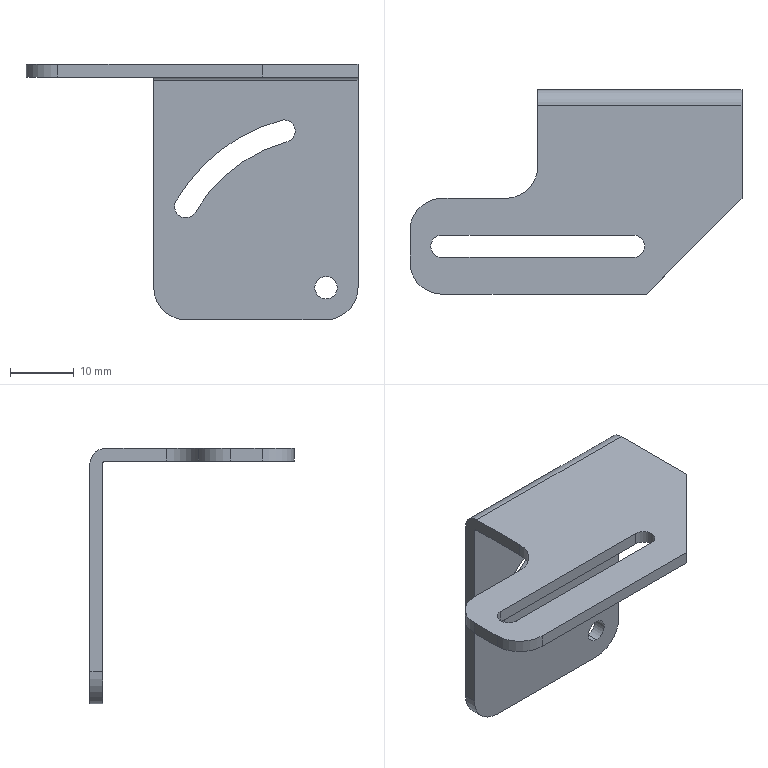Part | SolidWorks | features ICE 4, Fillet 3, Chamfer 1, Extrusion 1, HoleWzd 1 | 1 solid | 30 faces | box 52 x 32 x 40 mm | volume 4374 mm3 | cylinder 17 | plane 13 | commonest cylinder face diameters 3.5 x8 10 x5 1 x1 5 x1 47.3 x1 54.3 x1
STEP:
#1=CARTESIAN_POINT('',(20.879,-10.,-22.156));
#2=VERTEX_POINT('',#1);
#3=CARTESIAN_POINT('',(20.426,-10.,-18.715));
#4=VERTEX_POINT('',#3);
#5=CARTESIAN_POINT('',(20.426,-10.,-20.465));
#6=DIRECTION('',(0.,-1.,0.));
#7=DIRECTION('',(0.,0.,1.));
#8=AXIS2_PLACEMENT_3D('',#5,#6,#7);
#9=CIRCLE('',#8,1.75);
#10=EDGE_CURVE('',#2,#4,#9,.T.);
#11=ORIENTED_EDGE('',*,*,#10,.T.);
#12=CARTESIAN_POINT('',(20.426,-8.,-18.715));
#13=VERTEX_POINT('',#12);
#14=CARTESIAN_POINT('',(20.426,-40.001,-18.715));
#15=DIRECTION('',(0.,1.,0.));
#16=VECTOR('',#15,1000.);
#17=LINE('',#14,#16);
#18=EDGE_CURVE('',#4,#13,#17,.T.);
#19=ORIENTED_EDGE('',*,*,#18,.T.);
#20=CARTESIAN_POINT('',(20.879,-8.,-22.156));
#21=VERTEX_POINT('',#20);
#22=CARTESIAN_POINT('',(20.426,-8.,-20.465));
#23=DIRECTION('',(0.,1.,0.));
#24=DIRECTION('',(0.,0.,1.));
#25=AXIS2_PLACEMENT_3D('',#22,#23,#24);
#26=CIRCLE('',#25,1.75);
#27=EDGE_CURVE('',#13,#21,#26,.T.);
#28=ORIENTED_EDGE('',*,*,#27,.T.);
#29=CARTESIAN_POINT('',(20.879,-40.001,-22.156));
#30=DIRECTION('',(0.,1.,0.));
#31=VECTOR('',#30,1000.);
#32=LINE('',#29,#31);
#33=EDGE_CURVE('',#2,#21,#32,.T.);
#34=ORIENTED_EDGE('',*,*,#33,.F.);
#35=EDGE_LOOP('',(#11,#19,#28,#34));
#36=FACE_OUTER_BOUND('',#35,.T.);
#37=CARTESIAN_POINT('',(20.426,-40.001,-20.465));
#38=DIRECTION('',(0.,1.,0.));
#39=DIRECTION('',(0.,0.,1.));
#40=AXIS2_PLACEMENT_3D('',#37,#38,#39);
#41=CYLINDRICAL_SURFACE('',#40,1.75);
#42=ADVANCED_FACE('',(#36),#41,.F.);
#43=CARTESIAN_POINT('',(5.003,-8.,-34.05));
#44=VERTEX_POINT('',#43);
#45=CARTESIAN_POINT('',(6.518,-8.,-33.175));
#46=VERTEX_POINT('',#45);
#47=CARTESIAN_POINT('',(5.003,-8.,-32.3));
#48=DIRECTION('',(0.,-1.,0.));
#49=DIRECTION('',(0.,0.,-1.));
#50=AXIS2_PLACEMENT_3D('',#47,#48,#49);
#51=CIRCLE('',#50,1.75);
#52=EDGE_CURVE('',#44,#46,#51,.T.);
#53=ORIENTED_EDGE('',*,*,#52,.F.);
#54=CARTESIAN_POINT('',(5.003,-10.,-34.05));
#55=VERTEX_POINT('',#54);
#56=CARTESIAN_POINT('',(5.003,-10.,-34.05));
#57=DIRECTION('',(0.,-1.,0.));
#58=VECTOR('',#57,1000.);
#59=LINE('',#56,#58);
#60=EDGE_CURVE('',#44,#55,#59,.T.);
#61=ORIENTED_EDGE('',*,*,#60,.T.);
#62=CARTESIAN_POINT('',(6.518,-10.,-33.175));
#63=VERTEX_POINT('',#62);
#64=CARTESIAN_POINT('',(5.003,-10.,-32.3));
#65=DIRECTION('',(0.,-1.,0.));
#66=DIRECTION('',(0.,0.,-1.));
#67=AXIS2_PLACEMENT_3D('',#64,#65,#66);
#68=CIRCLE('',#67,1.75);
#69=EDGE_CURVE('',#55,#63,#68,.T.);
#70=ORIENTED_EDGE('',*,*,#69,.T.);
#71=CARTESIAN_POINT('',(6.518,-9.,-33.175));
#72=DIRECTION('',(0.,-1.,0.));
#73=VECTOR('',#72,1000.);
#74=LINE('',#71,#73);
#75=EDGE_CURVE('',#46,#63,#74,.T.);
#76=ORIENTED_EDGE('',*,*,#75,.F.);
#77=EDGE_LOOP('',(#53,#61,#70,#76));
#78=FACE_OUTER_BOUND('',#77,.T.);
#79=CARTESIAN_POINT('',(5.003,-10.,-32.3));
#80=DIRECTION('',(0.,-1.,0.));
#81=DIRECTION('',(0.,0.,-1.));
#82=AXIS2_PLACEMENT_3D('',#79,#80,#81);
#83=CYLINDRICAL_SURFACE('',#82,1.75);
#84=ADVANCED_FACE('',(#78),#83,.F.);
#85=CARTESIAN_POINT('',(27.,-8.,-43.25));
#86=VERTEX_POINT('',#85);
#87=CARTESIAN_POINT('',(27.,-8.,-46.75));
#88=VERTEX_POINT('',#87);
#89=CARTESIAN_POINT('',(27.,-8.,-45.));
#90=DIRECTION('',(0.,-1.,0.));
#91=DIRECTION('',(0.,0.,-1.));
#92=AXIS2_PLACEMENT_3D('',#89,#90,#91);
#93=CIRCLE('',#92,1.75);
#94=EDGE_CURVE('',#86,#88,#93,.T.);
#95=ORIENTED_EDGE('',*,*,#94,.F.);
#96=CARTESIAN_POINT('',(27.,-10.,-43.25));
#97=VERTEX_POINT('',#96);
#98=CARTESIAN_POINT('',(27.,-10.,-43.25));
#99=DIRECTION('',(0.,-1.,0.));
#100=VECTOR('',#99,1000.);
#101=LINE('',#98,#100);
#102=EDGE_CURVE('',#86,#97,#101,.T.);
#103=ORIENTED_EDGE('',*,*,#102,.T.);
#104=CARTESIAN_POINT('',(27.,-10.,-46.75));
#105=VERTEX_POINT('',#104);
#106=CARTESIAN_POINT('',(27.,-10.,-45.));
#107=DIRECTION('',(0.,-1.,0.));
#108=DIRECTION('',(0.,0.,-1.));
#109=AXIS2_PLACEMENT_3D('',#106,#107,#108);
#110=CIRCLE('',#109,1.75);
#111=EDGE_CURVE('',#97,#105,#110,.T.);
#112=ORIENTED_EDGE('',*,*,#111,.T.);
#113=CARTESIAN_POINT('',(27.,-10.,-46.75));
#114=DIRECTION('',(0.,-1.,0.));
#115=VECTOR('',#114,1000.);
#116=LINE('',#113,#115);
#117=EDGE_CURVE('',#88,#105,#116,.T.);
#118=ORIENTED_EDGE('',*,*,#117,.F.);
#119=EDGE_LOOP('',(#95,#103,#112,#118));
#120=FACE_OUTER_BOUND('',#119,.T.);
#121=CARTESIAN_POINT('',(27.,-10.,-45.));
#122=DIRECTION('',(0.,-1.,0.));
#123=DIRECTION('',(0.,0.,-1.));
#124=AXIS2_PLACEMENT_3D('',#121,#122,#123);
#125=CYLINDRICAL_SURFACE('',#124,1.75);
#126=ADVANCED_FACE('',(#120),#125,.F.);
#127=CARTESIAN_POINT('',(27.,-8.,-45.));
#128=DIRECTION('',(0.,-1.,0.));
#129=DIRECTION('',(0.,0.,1.));
#130=AXIS2_PLACEMENT_3D('',#127,#128,#129);
#131=CIRCLE('',#130,23.65);
#132=EDGE_CURVE('',#21,#46,#131,.T.);
#133=ORIENTED_EDGE('',*,*,#132,.F.);
#134=ORIENTED_EDGE('',*,*,#27,.F.);
#135=CARTESIAN_POINT('',(19.973,-8.,-18.775));
#136=VERTEX_POINT('',#135);
#137=CARTESIAN_POINT('',(20.426,-8.,-20.465));
#138=DIRECTION('',(0.,1.,0.));
#139=DIRECTION('',(0.,0.,1.));
#140=AXIS2_PLACEMENT_3D('',#137,#138,#139);
#141=CIRCLE('',#140,1.75);
#142=EDGE_CURVE('',#136,#13,#141,.T.);
#143=ORIENTED_EDGE('',*,*,#142,.F.);
#144=CARTESIAN_POINT('',(3.487,-8.,-31.425));
#145=VERTEX_POINT('',#144);
#146=CARTESIAN_POINT('',(27.,-8.,-45.));
#147=DIRECTION('',(0.,1.,0.));
#148=DIRECTION('',(0.,0.,1.));
#149=AXIS2_PLACEMENT_3D('',#146,#147,#148);
#150=CIRCLE('',#149,27.15);
#151=EDGE_CURVE('',#145,#136,#150,.T.);
#152=ORIENTED_EDGE('',*,*,#151,.F.);
#153=CARTESIAN_POINT('',(5.003,-8.,-32.3));
#154=DIRECTION('',(0.,-1.,0.));
#155=DIRECTION('',(0.,0.,-1.));
#156=AXIS2_PLACEMENT_3D('',#153,#154,#155);
#157=CIRCLE('',#156,1.75);
#158=EDGE_CURVE('',#145,#44,#157,.T.);
#159=ORIENTED_EDGE('',*,*,#158,.T.);
#160=ORIENTED_EDGE('',*,*,#52,.T.);
#161=EDGE_LOOP('',(#133,#134,#143,#152,#159,#160));
#162=FACE_BOUND('',#161,.T.);
#163=CARTESIAN_POINT('',(27.,-8.,-45.));
#164=DIRECTION('',(0.,-1.,0.));
#165=DIRECTION('',(0.,0.,-1.));
#166=AXIS2_PLACEMENT_3D('',#163,#164,#165);
#167=CIRCLE('',#166,1.75);
#168=EDGE_CURVE('',#88,#86,#167,.T.);
#169=ORIENTED_EDGE('',*,*,#168,.T.);
#170=ORIENTED_EDGE('',*,*,#94,.T.);
#171=EDGE_LOOP('',(#169,#170));
#172=FACE_BOUND('',#171,.T.);
#173=CARTESIAN_POINT('',(27.,-8.,-50.));
#174=VERTEX_POINT('',#173);
#175=CARTESIAN_POINT('',(5.,-8.,-50.));
#176=VERTEX_POINT('',#175);
#177=CARTESIAN_POINT('',(32.,-8.,-50.));
#178=DIRECTION('',(-1.,0.,0.));
#179=VECTOR('',#178,1000.);
#180=LINE('',#177,#179);
#181=EDGE_CURVE('',#174,#176,#180,.T.);
#182=ORIENTED_EDGE('',*,*,#181,.T.);
#183=CARTESIAN_POINT('',(0.,-8.,-45.));
#184=VERTEX_POINT('',#183);
#185=CARTESIAN_POINT('',(5.,-8.,-45.));
#186=DIRECTION('',(0.,1.,0.));
#187=DIRECTION('',(0.,0.,1.));
#188=AXIS2_PLACEMENT_3D('',#185,#186,#187);
#189=CIRCLE('',#188,5.);
#190=EDGE_CURVE('',#176,#184,#189,.T.);
#191=ORIENTED_EDGE('',*,*,#190,.T.);
#192=CARTESIAN_POINT('',(0.,-8.,-12.5));
#193=VERTEX_POINT('',#192);
#194=CARTESIAN_POINT('',(0.,-8.,-10.));
#195=DIRECTION('',(0.,0.,-1.));
#196=VECTOR('',#195,1000.);
#197=LINE('',#194,#196);
#198=EDGE_CURVE('',#193,#184,#197,.T.);
#199=ORIENTED_EDGE('',*,*,#198,.F.);
#200=CARTESIAN_POINT('',(32.,-8.,-12.5));
#201=VERTEX_POINT('',#200);
#202=CARTESIAN_POINT('',(32.,-8.,-12.5));
#203=DIRECTION('',(1.,0.,0.));
#204=VECTOR('',#203,1000.);
#205=LINE('',#202,#204);
#206=EDGE_CURVE('',#193,#201,#205,.T.);
#207=ORIENTED_EDGE('',*,*,#206,.T.);
#208=CARTESIAN_POINT('',(32.,-8.,-45.));
#209=VERTEX_POINT('',#208);
#210=CARTESIAN_POINT('',(32.,-8.,-10.));
#211=DIRECTION('',(0.,0.,-1.));
#212=VECTOR('',#211,1000.);
#213=LINE('',#210,#212);
#214=EDGE_CURVE('',#201,#209,#213,.T.);
#215=ORIENTED_EDGE('',*,*,#214,.T.);
#216=CARTESIAN_POINT('',(27.,-8.,-45.));
#217=DIRECTION('',(0.,1.,0.));
#218=DIRECTION('',(0.,0.,1.));
#219=AXIS2_PLACEMENT_3D('',#216,#217,#218);
#220=CIRCLE('',#219,5.);
#221=EDGE_CURVE('',#209,#174,#220,.T.);
#222=ORIENTED_EDGE('',*,*,#221,.T.);
#223=EDGE_LOOP('',(#182,#191,#199,#207,#215,#222));
#224=FACE_OUTER_BOUND('',#223,.T.);
#225=CARTESIAN_POINT('',(32.,-8.,-10.));
#226=DIRECTION('',(0.,1.,0.));
#227=DIRECTION('',(0.,0.,1.));
#228=AXIS2_PLACEMENT_3D('',#225,#226,#227);
#229=PLANE('',#228);
#230=ADVANCED_FACE('',(#162,#172,#224),#229,.T.);
#231=CARTESIAN_POINT('',(15.,-34.25,-10.));
#232=VERTEX_POINT('',#231);
#233=CARTESIAN_POINT('',(15.,-30.75,-10.));
#234=VERTEX_POINT('',#233);
#235=CARTESIAN_POINT('',(15.,-32.5,-10.));
#236=DIRECTION('',(0.,0.,1.));
#237=DIRECTION('',(0.,-1.,0.));
#238=AXIS2_PLACEMENT_3D('',#235,#236,#237);
#239=CIRCLE('',#238,1.75);
#240=EDGE_CURVE('',#232,#234,#239,.T.);
#241=ORIENTED_EDGE('',*,*,#240,.F.);
#242=CARTESIAN_POINT('',(-15.,-34.25,-10.));
#243=VERTEX_POINT('',#242);
#244=CARTESIAN_POINT('',(32.,-34.25,-10.));
#245=DIRECTION('',(1.,0.,0.));
#246=VECTOR('',#245,1000.);
#247=LINE('',#244,#246);
#248=EDGE_CURVE('',#243,#232,#247,.T.);
#249=ORIENTED_EDGE('',*,*,#248,.F.);
#250=CARTESIAN_POINT('',(-15.,-30.75,-10.));
#251=VERTEX_POINT('',#250);
#252=CARTESIAN_POINT('',(-15.,-32.5,-10.));
#253=DIRECTION('',(0.,0.,1.));
#254=DIRECTION('',(0.,-1.,0.));
#255=AXIS2_PLACEMENT_3D('',#252,#253,#254);
#256=CIRCLE('',#255,1.75);
#257=EDGE_CURVE('',#251,#243,#256,.T.);
#258=ORIENTED_EDGE('',*,*,#257,.F.);
#259=CARTESIAN_POINT('',(32.,-30.75,-10.));
#260=DIRECTION('',(-1.,0.,0.));
#261=VECTOR('',#260,1000.);
#262=LINE('',#259,#261);
#263=EDGE_CURVE('',#234,#251,#262,.T.);
#264=ORIENTED_EDGE('',*,*,#263,.F.);
#265=EDGE_LOOP('',(#241,#249,#258,#264));
#266=FACE_BOUND('',#265,.T.);
#267=CARTESIAN_POINT('',(-20.,-35.,-10.));
#268=VERTEX_POINT('',#267);
#269=CARTESIAN_POINT('',(-20.,-30.,-10.));
#270=VERTEX_POINT('',#269);
#271=CARTESIAN_POINT('',(-20.,-40.,-10.));
#272=DIRECTION('',(0.,1.,0.));
#273=VECTOR('',#272,1000.);
#274=LINE('',#271,#273);
#275=EDGE_CURVE('',#268,#270,#274,.T.);
#276=ORIENTED_EDGE('',*,*,#275,.F.);
#277=CARTESIAN_POINT('',(-15.,-40.,-10.));
#278=VERTEX_POINT('',#277);
#279=CARTESIAN_POINT('',(-15.,-35.,-10.));
#280=DIRECTION('',(0.,0.,1.));
#281=DIRECTION('',(0.,-1.,0.));
#282=AXIS2_PLACEMENT_3D('',#279,#280,#281);
#283=CIRCLE('',#282,5.);
#284=EDGE_CURVE('',#268,#278,#283,.T.);
#285=ORIENTED_EDGE('',*,*,#284,.T.);
#286=CARTESIAN_POINT('',(17.,-40.,-10.));
#287=VERTEX_POINT('',#286);
#288=CARTESIAN_POINT('',(32.,-40.,-10.));
#289=DIRECTION('',(-1.,0.,0.));
#290=VECTOR('',#289,1000.);
#291=LINE('',#288,#290);
#292=EDGE_CURVE('',#287,#278,#291,.T.);
#293=ORIENTED_EDGE('',*,*,#292,.F.);
#294=CARTESIAN_POINT('',(32.,-25.,-10.));
#295=VERTEX_POINT('',#294);
#296=CARTESIAN_POINT('',(24.5,-32.5,-10.));
#297=DIRECTION('',(0.7071,0.7071,0.));
#298=VECTOR('',#297,1000.);
#299=LINE('',#296,#298);
#300=EDGE_CURVE('',#287,#295,#299,.T.);
#301=ORIENTED_EDGE('',*,*,#300,.T.);
#302=CARTESIAN_POINT('',(32.,-10.5,-10.));
#303=VERTEX_POINT('',#302);
#304=CARTESIAN_POINT('',(32.,-40.,-10.));
#305=DIRECTION('',(0.,1.,0.));
#306=VECTOR('',#305,1000.);
#307=LINE('',#304,#306);
#308=EDGE_CURVE('',#295,#303,#307,.T.);
#309=ORIENTED_EDGE('',*,*,#308,.T.);
#310=CARTESIAN_POINT('',(0.,-10.5,-10.));
#311=VERTEX_POINT('',#310);
#312=CARTESIAN_POINT('',(32.,-10.5,-10.));
#313=DIRECTION('',(-1.,0.,0.));
#314=VECTOR('',#313,1000.);
#315=LINE('',#312,#314);
#316=EDGE_CURVE('',#303,#311,#315,.T.);
#317=ORIENTED_EDGE('',*,*,#316,.T.);
#318=CARTESIAN_POINT('',(0.,-20.,-10.));
#319=VERTEX_POINT('',#318);
#320=CARTESIAN_POINT('',(0.,-40.,-10.));
#321=DIRECTION('',(0.,1.,0.));
#322=VECTOR('',#321,1000.);
#323=LINE('',#320,#322);
#324=EDGE_CURVE('',#319,#311,#323,.T.);
#325=ORIENTED_EDGE('',*,*,#324,.F.);
#326=CARTESIAN_POINT('',(-5.,-25.,-10.));
#327=VERTEX_POINT('',#326);
#328=CARTESIAN_POINT('',(-5.,-20.,-10.));
#329=DIRECTION('',(0.,0.,-1.));
#330=DIRECTION('',(0.,-1.,0.));
#331=AXIS2_PLACEMENT_3D('',#328,#329,#330);
#332=CIRCLE('',#331,5.);
#333=EDGE_CURVE('',#319,#327,#332,.T.);
#334=ORIENTED_EDGE('',*,*,#333,.T.);
#335=CARTESIAN_POINT('',(-15.,-25.,-10.));
#336=VERTEX_POINT('',#335);
#337=CARTESIAN_POINT('',(-20.,-25.,-10.));
#338=DIRECTION('',(1.,0.,0.));
#339=VECTOR('',#338,1000.);
#340=LINE('',#337,#339);
#341=EDGE_CURVE('',#336,#327,#340,.T.);
#342=ORIENTED_EDGE('',*,*,#341,.F.);
#343=CARTESIAN_POINT('',(-15.,-30.,-10.));
#344=DIRECTION('',(0.,0.,1.));
#345=DIRECTION('',(0.,-1.,0.));
#346=AXIS2_PLACEMENT_3D('',#343,#344,#345);
#347=CIRCLE('',#346,5.);
#348=EDGE_CURVE('',#336,#270,#347,.T.);
#349=ORIENTED_EDGE('',*,*,#348,.T.);
#350=EDGE_LOOP('',(#276,#285,#293,#301,#309,#317,#325,#334,#342,#349));
#351=FACE_OUTER_BOUND('',#350,.T.);
#352=CARTESIAN_POINT('',(32.,-40.,-10.));
#353=DIRECTION('',(0.,0.,1.));
#354=DIRECTION('',(0.,-1.,0.));
#355=AXIS2_PLACEMENT_3D('',#352,#353,#354);
#356=PLANE('',#355);
#357=ADVANCED_FACE('',(#266,#351),#356,.T.);
#358=ORIENTED_EDGE('',*,*,#292,.T.);
#359=CARTESIAN_POINT('',(-15.,-40.,-12.));
#360=VERTEX_POINT('',#359);
#361=CARTESIAN_POINT('',(-15.,-40.,-50.));
#362=DIRECTION('',(0.,0.,-1.));
#363=VECTOR('',#362,1000.);
#364=LINE('',#361,#363);
#365=EDGE_CURVE('',#278,#360,#364,.T.);
#366=ORIENTED_EDGE('',*,*,#365,.T.);
#367=CARTESIAN_POINT('',(17.,-40.,-12.));
#368=VERTEX_POINT('',#367);
#369=CARTESIAN_POINT('',(32.,-40.,-12.));
#370=DIRECTION('',(-1.,0.,0.));
#371=VECTOR('',#370,1000.);
#372=LINE('',#369,#371);
#373=EDGE_CURVE('',#368,#360,#372,.T.);
#374=ORIENTED_EDGE('',*,*,#373,.F.);
#375=CARTESIAN_POINT('',(17.,-40.,-10.));
#376=DIRECTION('',(0.,0.,1.));
#377=VECTOR('',#376,1000.);
#378=LINE('',#375,#377);
#379=EDGE_CURVE('',#368,#287,#378,.T.);
#380=ORIENTED_EDGE('',*,*,#379,.T.);
#381=EDGE_LOOP('',(#358,#366,#374,#380));
#382=FACE_OUTER_BOUND('',#381,.T.);
#383=CARTESIAN_POINT('',(32.,-40.,-50.));
#384=DIRECTION('',(0.,-1.,0.));
#385=DIRECTION('',(0.,0.,-1.));
#386=AXIS2_PLACEMENT_3D('',#383,#384,#385);
#387=PLANE('',#386);
#388=ADVANCED_FACE('',(#382),#387,.T.);
#389=CARTESIAN_POINT('',(5.,-10.,-50.));
#390=VERTEX_POINT('',#389);
#391=CARTESIAN_POINT('',(27.,-10.,-50.));
#392=VERTEX_POINT('',#391);
#393=CARTESIAN_POINT('',(32.,-10.,-50.));
#394=DIRECTION('',(1.,0.,0.));
#395=VECTOR('',#394,1000.);
#396=LINE('',#393,#395);
#397=EDGE_CURVE('',#390,#392,#396,.T.);
#398=ORIENTED_EDGE('',*,*,#397,.F.);
#399=CARTESIAN_POINT('',(5.,-8.,-50.));
#400=DIRECTION('',(0.,1.,0.));
#401=VECTOR('',#400,1000.);
#402=LINE('',#399,#401);
#403=EDGE_CURVE('',#390,#176,#402,.T.);
#404=ORIENTED_EDGE('',*,*,#403,.T.);
#405=ORIENTED_EDGE('',*,*,#181,.F.);
#406=CARTESIAN_POINT('',(27.,-10.,-50.));
#407=DIRECTION('',(0.,-1.,0.));
#408=VECTOR('',#407,1000.);
#409=LINE('',#406,#408);
#410=EDGE_CURVE('',#174,#392,#409,.T.);
#411=ORIENTED_EDGE('',*,*,#410,.T.);
#412=EDGE_LOOP('',(#398,#404,#405,#411));
#413=FACE_OUTER_BOUND('',#412,.T.);
#414=CARTESIAN_POINT('',(32.,-8.,-50.));
#415=DIRECTION('',(0.,0.,-1.));
#416=DIRECTION('',(-1.,0.,0.));
#417=AXIS2_PLACEMENT_3D('',#414,#415,#416);
#418=PLANE('',#417);
#419=ADVANCED_FACE('',(#413),#418,.T.);
#420=CARTESIAN_POINT('',(32.,-10.,-45.));
#421=VERTEX_POINT('',#420);
#422=CARTESIAN_POINT('',(32.,-10.,-12.5));
#423=VERTEX_POINT('',#422);
#424=CARTESIAN_POINT('',(32.,-10.,-57.59));
#425=DIRECTION('',(0.,0.,1.));
#426=VECTOR('',#425,1000.);
#427=LINE('',#424,#426);
#428=EDGE_CURVE('',#421,#423,#427,.T.);
#429=ORIENTED_EDGE('',*,*,#428,.F.);
#430=CARTESIAN_POINT('',(32.,-8.,-45.));
#431=DIRECTION('',(0.,1.,0.));
#432=VECTOR('',#431,1000.);
#433=LINE('',#430,#432);
#434=EDGE_CURVE('',#421,#209,#433,.T.);
#435=ORIENTED_EDGE('',*,*,#434,.T.);
#436=ORIENTED_EDGE('',*,*,#214,.F.);
#437=CARTESIAN_POINT('',(32.,-10.5,-12.5));
#438=DIRECTION('',(1.,0.,0.));
#439=DIRECTION('',(0.,0.,1.));
#440=AXIS2_PLACEMENT_3D('',#437,#438,#439);
#441=CIRCLE('',#440,2.5);
#442=EDGE_CURVE('',#201,#303,#441,.T.);
#443=ORIENTED_EDGE('',*,*,#442,.T.);
#444=ORIENTED_EDGE('',*,*,#308,.F.);
#445=CARTESIAN_POINT('',(32.,-25.,-12.));
#446=VERTEX_POINT('',#445);
#447=CARTESIAN_POINT('',(32.,-25.,-12.));
#448=DIRECTION('',(0.,0.,-1.));
#449=VECTOR('',#448,1000.);
#450=LINE('',#447,#449);
#451=EDGE_CURVE('',#295,#446,#450,.T.);
#452=ORIENTED_EDGE('',*,*,#451,.T.);
#453=CARTESIAN_POINT('',(32.,-10.5,-12.));
#454=VERTEX_POINT('',#453);
#455=CARTESIAN_POINT('',(32.,-10.,-12.));
#456=DIRECTION('',(0.,-1.,0.));
#457=VECTOR('',#456,1000.);
#458=LINE('',#455,#457);
#459=EDGE_CURVE('',#454,#446,#458,.T.);
#460=ORIENTED_EDGE('',*,*,#459,.F.);
#461=CARTESIAN_POINT('',(32.,-10.5,-12.5));
#462=DIRECTION('',(-1.,0.,0.));
#463=DIRECTION('',(0.,0.,1.));
#464=AXIS2_PLACEMENT_3D('',#461,#462,#463);
#465=CIRCLE('',#464,0.5);
#466=EDGE_CURVE('',#454,#423,#465,.T.);
#467=ORIENTED_EDGE('',*,*,#466,.T.);
#468=EDGE_LOOP('',(#429,#435,#436,#443,#444,#452,#460,#467));
#469=FACE_OUTER_BOUND('',#468,.T.);
#470=CARTESIAN_POINT('',(32.,0.,0.));
#471=DIRECTION('',(-1.,0.,0.));
#472=DIRECTION('',(0.,0.,1.));
#473=AXIS2_PLACEMENT_3D('',#470,#471,#472);
#474=PLANE('',#473);
#475=ADVANCED_FACE('',(#469),#474,.F.);
#476=CARTESIAN_POINT('',(0.,-10.5,-12.));
#477=VERTEX_POINT('',#476);
#478=CARTESIAN_POINT('',(0.,-20.,-12.));
#479=VERTEX_POINT('',#478);
#480=CARTESIAN_POINT('',(0.,-10.,-12.));
#481=DIRECTION('',(0.,-1.,0.));
#482=VECTOR('',#481,1000.);
#483=LINE('',#480,#482);
#484=EDGE_CURVE('',#477,#479,#483,.T.);
#485=ORIENTED_EDGE('',*,*,#484,.T.);
#486=CARTESIAN_POINT('',(0.,-20.,0.));
#487=DIRECTION('',(0.,0.,1.));
#488=VECTOR('',#487,1000.);
#489=LINE('',#486,#488);
#490=EDGE_CURVE('',#479,#319,#489,.T.);
#491=ORIENTED_EDGE('',*,*,#490,.T.);
#492=ORIENTED_EDGE('',*,*,#324,.T.);
#493=CARTESIAN_POINT('',(0.,-10.5,-12.5));
#494=DIRECTION('',(-1.,0.,0.));
#495=DIRECTION('',(0.,0.,1.));
#496=AXIS2_PLACEMENT_3D('',#493,#494,#495);
#497=CIRCLE('',#496,2.5);
#498=EDGE_CURVE('',#311,#193,#497,.T.);
#499=ORIENTED_EDGE('',*,*,#498,.T.);
#500=ORIENTED_EDGE('',*,*,#198,.T.);
#501=CARTESIAN_POINT('',(0.,-10.,-45.));
#502=VERTEX_POINT('',#501);
#503=CARTESIAN_POINT('',(0.,0.,-45.));
#504=DIRECTION('',(0.,-1.,0.));
#505=VECTOR('',#504,1000.);
#506=LINE('',#503,#505);
#507=EDGE_CURVE('',#184,#502,#506,.T.);
#508=ORIENTED_EDGE('',*,*,#507,.T.);
#509=CARTESIAN_POINT('',(0.,-10.,-12.5));
#510=VERTEX_POINT('',#509);
#511=CARTESIAN_POINT('',(0.,-10.,0.));
#512=DIRECTION('',(0.,0.,-1.));
#513=VECTOR('',#512,1000.);
#514=LINE('',#511,#513);
#515=EDGE_CURVE('',#510,#502,#514,.T.);
#516=ORIENTED_EDGE('',*,*,#515,.F.);
#517=CARTESIAN_POINT('',(0.,-10.5,-12.5));
#518=DIRECTION('',(1.,0.,0.));
#519=DIRECTION('',(0.,0.,1.));
#520=AXIS2_PLACEMENT_3D('',#517,#518,#519);
#521=CIRCLE('',#520,0.5);
#522=EDGE_CURVE('',#510,#477,#521,.T.);
#523=ORIENTED_EDGE('',*,*,#522,.T.);
#524=EDGE_LOOP('',(#485,#491,#492,#499,#500,#508,#516,#523));
#525=FACE_OUTER_BOUND('',#524,.T.);
#526=CARTESIAN_POINT('',(0.,0.,0.));
#527=DIRECTION('',(-1.,0.,0.));
#528=DIRECTION('',(0.,0.,1.));
#529=AXIS2_PLACEMENT_3D('',#526,#527,#528);
#530=PLANE('',#529);
#531=ADVANCED_FACE('',(#525),#530,.T.);
#532=CARTESIAN_POINT('',(15.,-34.25,-12.));
#533=VERTEX_POINT('',#532);
#534=CARTESIAN_POINT('',(-15.,-34.25,-12.));
#535=VERTEX_POINT('',#534);
#536=CARTESIAN_POINT('',(15.,-34.25,-12.));
#537=DIRECTION('',(-1.,0.,0.));
#538=VECTOR('',#537,1000.);
#539=LINE('',#536,#538);
#540=EDGE_CURVE('',#533,#535,#539,.T.);
#541=ORIENTED_EDGE('',*,*,#540,.F.);
#542=CARTESIAN_POINT('',(15.,-30.75,-12.));
#543=VERTEX_POINT('',#542);
#544=CARTESIAN_POINT('',(15.,-32.5,-12.));
#545=DIRECTION('',(0.,0.,-1.));
#546=DIRECTION('',(0.,1.,0.));
#547=AXIS2_PLACEMENT_3D('',#544,#545,#546);
#548=CIRCLE('',#547,1.75);
#549=EDGE_CURVE('',#543,#533,#548,.T.);
#550=ORIENTED_EDGE('',*,*,#549,.F.);
#551=CARTESIAN_POINT('',(-15.,-30.75,-12.));
#552=VERTEX_POINT('',#551);
#553=CARTESIAN_POINT('',(15.,-30.75,-12.));
#554=DIRECTION('',(1.,0.,0.));
#555=VECTOR('',#554,1000.);
#556=LINE('',#553,#555);
#557=EDGE_CURVE('',#552,#543,#556,.T.);
#558=ORIENTED_EDGE('',*,*,#557,.F.);
#559=CARTESIAN_POINT('',(-15.,-32.5,-12.));
#560=DIRECTION('',(0.,0.,-1.));
#561=DIRECTION('',(0.,1.,0.));
#562=AXIS2_PLACEMENT_3D('',#559,#560,#561);
#563=CIRCLE('',#562,1.75);
#564=EDGE_CURVE('',#535,#552,#563,.T.);
#565=ORIENTED_EDGE('',*,*,#564,.F.);
#566=EDGE_LOOP('',(#541,#550,#558,#565));
#567=FACE_BOUND('',#566,.T.);
#568=ORIENTED_EDGE('',*,*,#373,.T.);
#569=CARTESIAN_POINT('',(-20.,-35.,-12.));
#570=VERTEX_POINT('',#569);
#571=CARTESIAN_POINT('',(-15.,-35.,-12.));
#572=DIRECTION('',(0.,0.,-1.));
#573=DIRECTION('',(0.,-1.,0.));
#574=AXIS2_PLACEMENT_3D('',#571,#572,#573);
#575=CIRCLE('',#574,5.);
#576=EDGE_CURVE('',#360,#570,#575,.T.);
#577=ORIENTED_EDGE('',*,*,#576,.T.);
#578=CARTESIAN_POINT('',(-20.,-30.,-12.));
#579=VERTEX_POINT('',#578);
#580=CARTESIAN_POINT('',(-20.,-40.,-12.));
#581=DIRECTION('',(0.,-1.,0.));
#582=VECTOR('',#581,1000.);
#583=LINE('',#580,#582);
#584=EDGE_CURVE('',#579,#570,#583,.T.);
#585=ORIENTED_EDGE('',*,*,#584,.F.);
#586=CARTESIAN_POINT('',(-15.,-25.,-12.));
#587=VERTEX_POINT('',#586);
#588=CARTESIAN_POINT('',(-15.,-30.,-12.));
#589=DIRECTION('',(0.,0.,-1.));
#590=DIRECTION('',(0.,-1.,0.));
#591=AXIS2_PLACEMENT_3D('',#588,#589,#590);
#592=CIRCLE('',#591,5.);
#593=EDGE_CURVE('',#579,#587,#592,.T.);
#594=ORIENTED_EDGE('',*,*,#593,.T.);
#595=CARTESIAN_POINT('',(-5.,-25.,-12.));
#596=VERTEX_POINT('',#595);
#597=CARTESIAN_POINT('',(-20.,-25.,-12.));
#598=DIRECTION('',(1.,0.,0.));
#599=VECTOR('',#598,1000.);
#600=LINE('',#597,#599);
#601=EDGE_CURVE('',#587,#596,#600,.T.);
#602=ORIENTED_EDGE('',*,*,#601,.T.);
#603=CARTESIAN_POINT('',(-5.,-20.,-12.));
#604=DIRECTION('',(0.,0.,1.));
#605=DIRECTION('',(0.,-1.,0.));
#606=AXIS2_PLACEMENT_3D('',#603,#604,#605);
#607=CIRCLE('',#606,5.);
#608=EDGE_CURVE('',#596,#479,#607,.T.);
#609=ORIENTED_EDGE('',*,*,#608,.T.);
#610=ORIENTED_EDGE('',*,*,#484,.F.);
#611=CARTESIAN_POINT('',(32.,-10.5,-12.));
#612=DIRECTION('',(1.,0.,0.));
#613=VECTOR('',#612,1000.);
#614=LINE('',#611,#613);
#615=EDGE_CURVE('',#477,#454,#614,.T.);
#616=ORIENTED_EDGE('',*,*,#615,.T.);
#617=ORIENTED_EDGE('',*,*,#459,.T.);
#618=CARTESIAN_POINT('',(17.,-40.,-12.));
#619=DIRECTION('',(-0.7071,-0.7071,0.));
#620=VECTOR('',#619,1000.);
#621=LINE('',#618,#620);
#622=EDGE_CURVE('',#446,#368,#621,.T.);
#623=ORIENTED_EDGE('',*,*,#622,.T.);
#624=EDGE_LOOP('',(#568,#577,#585,#594,#602,#609,#610,#616,#617,#623));
#625=FACE_OUTER_BOUND('',#624,.T.);
#626=CARTESIAN_POINT('',(0.,-10.,-12.));
#627=DIRECTION('',(0.,0.,1.));
#628=DIRECTION('',(0.,-1.,0.));
#629=AXIS2_PLACEMENT_3D('',#626,#627,#628);
#630=PLANE('',#629);
#631=ADVANCED_FACE('',(#567,#625),#630,.F.);
#632=ORIENTED_EDGE('',*,*,#10,.F.);
#633=CARTESIAN_POINT('',(27.,-10.,-45.));
#634=DIRECTION('',(0.,1.,0.));
#635=DIRECTION('',(0.,0.,1.));
#636=AXIS2_PLACEMENT_3D('',#633,#634,#635);
#637=CIRCLE('',#636,23.65);
#638=EDGE_CURVE('',#63,#2,#637,.T.);
#639=ORIENTED_EDGE('',*,*,#638,.F.);
#640=ORIENTED_EDGE('',*,*,#69,.F.);
#641=CARTESIAN_POINT('',(3.487,-10.,-31.425));
#642=VERTEX_POINT('',#641);
#643=CARTESIAN_POINT('',(5.003,-10.,-32.3));
#644=DIRECTION('',(0.,-1.,0.));
#645=DIRECTION('',(0.,0.,-1.));
#646=AXIS2_PLACEMENT_3D('',#643,#644,#645);
#647=CIRCLE('',#646,1.75);
#648=EDGE_CURVE('',#642,#55,#647,.T.);
#649=ORIENTED_EDGE('',*,*,#648,.F.);
#650=CARTESIAN_POINT('',(19.973,-10.,-18.775));
#651=VERTEX_POINT('',#650);
#652=CARTESIAN_POINT('',(27.,-10.,-45.));
#653=DIRECTION('',(0.,-1.,0.));
#654=DIRECTION('',(0.,0.,1.));
#655=AXIS2_PLACEMENT_3D('',#652,#653,#654);
#656=CIRCLE('',#655,27.15);
#657=EDGE_CURVE('',#651,#642,#656,.T.);
#658=ORIENTED_EDGE('',*,*,#657,.F.);
#659=CARTESIAN_POINT('',(20.426,-10.,-20.465));
#660=DIRECTION('',(0.,-1.,0.));
#661=DIRECTION('',(0.,0.,1.));
#662=AXIS2_PLACEMENT_3D('',#659,#660,#661);
#663=CIRCLE('',#662,1.75);
#664=EDGE_CURVE('',#4,#651,#663,.T.);
#665=ORIENTED_EDGE('',*,*,#664,.F.);
#666=EDGE_LOOP('',(#632,#639,#640,#649,#658,#665));
#667=FACE_BOUND('',#666,.T.);
#668=CARTESIAN_POINT('',(27.,-10.,-45.));
#669=DIRECTION('',(0.,-1.,0.));
#670=DIRECTION('',(0.,0.,-1.));
#671=AXIS2_PLACEMENT_3D('',#668,#669,#670);
#672=CIRCLE('',#671,1.75);
#673=EDGE_CURVE('',#105,#97,#672,.T.);
#674=ORIENTED_EDGE('',*,*,#673,.F.);
#675=ORIENTED_EDGE('',*,*,#111,.F.);
#676=EDGE_LOOP('',(#674,#675));
#677=FACE_BOUND('',#676,.T.);
#678=ORIENTED_EDGE('',*,*,#515,.T.);
#679=CARTESIAN_POINT('',(5.,-10.,-45.));
#680=DIRECTION('',(0.,-1.,0.));
#681=DIRECTION('',(0.,0.,1.));
#682=AXIS2_PLACEMENT_3D('',#679,#680,#681);
#683=CIRCLE('',#682,5.);
#684=EDGE_CURVE('',#502,#390,#683,.T.);
#685=ORIENTED_EDGE('',*,*,#684,.T.);
#686=ORIENTED_EDGE('',*,*,#397,.T.);
#687=CARTESIAN_POINT('',(27.,-10.,-45.));
#688=DIRECTION('',(0.,-1.,0.));
#689=DIRECTION('',(0.,0.,1.));
#690=AXIS2_PLACEMENT_3D('',#687,#688,#689);
#691=CIRCLE('',#690,5.);
#692=EDGE_CURVE('',#392,#421,#691,.T.);
#693=ORIENTED_EDGE('',*,*,#692,.T.);
#694=ORIENTED_EDGE('',*,*,#428,.T.);
#695=CARTESIAN_POINT('',(0.,-10.,-12.5));
#696=DIRECTION('',(-1.,0.,0.));
#697=VECTOR('',#696,1000.);
#698=LINE('',#695,#697);
#699=EDGE_CURVE('',#423,#510,#698,.T.);
#700=ORIENTED_EDGE('',*,*,#699,.T.);
#701=EDGE_LOOP('',(#678,#685,#686,#693,#694,#700));
#702=FACE_OUTER_BOUND('',#701,.T.);
#703=CARTESIAN_POINT('',(0.,-10.,-57.59));
#704=DIRECTION('',(0.,1.,0.));
#705=DIRECTION('',(0.,0.,1.));
#706=AXIS2_PLACEMENT_3D('',#703,#704,#705);
#707=PLANE('',#706);
#708=ADVANCED_FACE('',(#667,#677,#702),#707,.F.);
#709=ORIENTED_EDGE('',*,*,#102,.F.);
#710=ORIENTED_EDGE('',*,*,#168,.F.);
#711=ORIENTED_EDGE('',*,*,#117,.T.);
#712=ORIENTED_EDGE('',*,*,#673,.T.);
#713=EDGE_LOOP('',(#709,#710,#711,#712));
#714=FACE_OUTER_BOUND('',#713,.T.);
#715=CARTESIAN_POINT('',(27.,-10.,-45.));
#716=DIRECTION('',(0.,-1.,0.));
#717=DIRECTION('',(0.,0.,-1.));
#718=AXIS2_PLACEMENT_3D('',#715,#716,#717);
#719=CYLINDRICAL_SURFACE('',#718,1.75);
#720=ADVANCED_FACE('',(#714),#719,.F.);
#721=ORIENTED_EDGE('',*,*,#60,.F.);
#722=ORIENTED_EDGE('',*,*,#158,.F.);
#723=CARTESIAN_POINT('',(3.487,-9.,-31.425));
#724=DIRECTION('',(0.,-1.,0.));
#725=VECTOR('',#724,1000.);
#726=LINE('',#723,#725);
#727=EDGE_CURVE('',#145,#642,#726,.T.);
#728=ORIENTED_EDGE('',*,*,#727,.T.);
#729=ORIENTED_EDGE('',*,*,#648,.T.);
#730=EDGE_LOOP('',(#721,#722,#728,#729));
#731=FACE_OUTER_BOUND('',#730,.T.);
#732=CARTESIAN_POINT('',(5.003,-10.,-32.3));
#733=DIRECTION('',(0.,-1.,0.));
#734=DIRECTION('',(0.,0.,-1.));
#735=AXIS2_PLACEMENT_3D('',#732,#733,#734);
#736=CYLINDRICAL_SURFACE('',#735,1.75);
#737=ADVANCED_FACE('',(#731),#736,.F.);
#738=ORIENTED_EDGE('',*,*,#522,.F.);
#739=ORIENTED_EDGE('',*,*,#699,.F.);
#740=ORIENTED_EDGE('',*,*,#466,.F.);
#741=ORIENTED_EDGE('',*,*,#615,.F.);
#742=EDGE_LOOP('',(#738,#739,#740,#741));
#743=FACE_OUTER_BOUND('',#742,.T.);
#744=CARTESIAN_POINT('',(0.,-10.5,-12.5));
#745=DIRECTION('',(-1.,0.,0.));
#746=DIRECTION('',(0.,0.,1.));
#747=AXIS2_PLACEMENT_3D('',#744,#745,#746);
#748=CYLINDRICAL_SURFACE('',#747,0.5);
#749=ADVANCED_FACE('',(#743),#748,.F.);
#750=ORIENTED_EDGE('',*,*,#442,.F.);
#751=ORIENTED_EDGE('',*,*,#206,.F.);
#752=ORIENTED_EDGE('',*,*,#498,.F.);
#753=ORIENTED_EDGE('',*,*,#316,.F.);
#754=EDGE_LOOP('',(#750,#751,#752,#753));
#755=FACE_OUTER_BOUND('',#754,.T.);
#756=CARTESIAN_POINT('',(32.,-10.5,-12.5));
#757=DIRECTION('',(-1.,0.,0.));
#758=DIRECTION('',(0.,0.,1.));
#759=AXIS2_PLACEMENT_3D('',#756,#757,#758);
#760=CYLINDRICAL_SURFACE('',#759,2.5);
#761=ADVANCED_FACE('',(#755),#760,.T.);
#762=ORIENTED_EDGE('',*,*,#638,.T.);
#763=ORIENTED_EDGE('',*,*,#33,.T.);
#764=ORIENTED_EDGE('',*,*,#132,.T.);
#765=ORIENTED_EDGE('',*,*,#75,.T.);
#766=EDGE_LOOP('',(#762,#763,#764,#765));
#767=FACE_OUTER_BOUND('',#766,.T.);
#768=CARTESIAN_POINT('',(27.,-40.001,-45.));
#769=DIRECTION('',(0.,1.,0.));
#770=DIRECTION('',(0.,0.,1.));
#771=AXIS2_PLACEMENT_3D('',#768,#769,#770);
#772=CYLINDRICAL_SURFACE('',#771,23.65);
#773=ADVANCED_FACE('',(#767),#772,.T.);
#774=ORIENTED_EDGE('',*,*,#18,.F.);
#775=ORIENTED_EDGE('',*,*,#664,.T.);
#776=CARTESIAN_POINT('',(19.973,-40.001,-18.775));
#777=DIRECTION('',(0.,1.,0.));
#778=VECTOR('',#777,1000.);
#779=LINE('',#776,#778);
#780=EDGE_CURVE('',#651,#136,#779,.T.);
#781=ORIENTED_EDGE('',*,*,#780,.T.);
#782=ORIENTED_EDGE('',*,*,#142,.T.);
#783=EDGE_LOOP('',(#774,#775,#781,#782));
#784=FACE_OUTER_BOUND('',#783,.T.);
#785=CARTESIAN_POINT('',(20.426,-40.001,-20.465));
#786=DIRECTION('',(0.,1.,0.));
#787=DIRECTION('',(0.,0.,1.));
#788=AXIS2_PLACEMENT_3D('',#785,#786,#787);
#789=CYLINDRICAL_SURFACE('',#788,1.75);
#790=ADVANCED_FACE('',(#784),#789,.F.);
#791=ORIENTED_EDGE('',*,*,#657,.T.);
#792=ORIENTED_EDGE('',*,*,#727,.F.);
#793=ORIENTED_EDGE('',*,*,#151,.T.);
#794=ORIENTED_EDGE('',*,*,#780,.F.);
#795=EDGE_LOOP('',(#791,#792,#793,#794));
#796=FACE_OUTER_BOUND('',#795,.T.);
#797=CARTESIAN_POINT('',(27.,-40.001,-45.));
#798=DIRECTION('',(0.,1.,0.));
#799=DIRECTION('',(0.,0.,1.));
#800=AXIS2_PLACEMENT_3D('',#797,#798,#799);
#801=CYLINDRICAL_SURFACE('',#800,27.15);
#802=ADVANCED_FACE('',(#796),#801,.F.);
#803=ORIENTED_EDGE('',*,*,#341,.T.);
#804=CARTESIAN_POINT('',(-5.,-25.,-10.));
#805=DIRECTION('',(0.,0.,-1.));
#806=VECTOR('',#805,1000.);
#807=LINE('',#804,#806);
#808=EDGE_CURVE('',#327,#596,#807,.T.);
#809=ORIENTED_EDGE('',*,*,#808,.T.);
#810=ORIENTED_EDGE('',*,*,#601,.F.);
#811=CARTESIAN_POINT('',(-15.,-25.,-10.));
#812=DIRECTION('',(0.,0.,1.));
#813=VECTOR('',#812,1000.);
#814=LINE('',#811,#813);
#815=EDGE_CURVE('',#587,#336,#814,.T.);
#816=ORIENTED_EDGE('',*,*,#815,.T.);
#817=EDGE_LOOP('',(#803,#809,#810,#816));
#818=FACE_OUTER_BOUND('',#817,.T.);
#819=CARTESIAN_POINT('',(-20.,-25.,-10.));
#820=DIRECTION('',(0.,-1.,0.));
#821=DIRECTION('',(0.,0.,-1.));
#822=AXIS2_PLACEMENT_3D('',#819,#820,#821);
#823=PLANE('',#822);
#824=ADVANCED_FACE('',(#818),#823,.F.);
#825=ORIENTED_EDGE('',*,*,#584,.T.);
#826=CARTESIAN_POINT('',(-20.,-35.,0.));
#827=DIRECTION('',(0.,0.,1.));
#828=VECTOR('',#827,1000.);
#829=LINE('',#826,#828);
#830=EDGE_CURVE('',#570,#268,#829,.T.);
#831=ORIENTED_EDGE('',*,*,#830,.T.);
#832=ORIENTED_EDGE('',*,*,#275,.T.);
#833=CARTESIAN_POINT('',(-20.,-30.,-12.));
#834=DIRECTION('',(0.,0.,-1.));
#835=VECTOR('',#834,1000.);
#836=LINE('',#833,#835);
#837=EDGE_CURVE('',#270,#579,#836,.T.);
#838=ORIENTED_EDGE('',*,*,#837,.T.);
#839=EDGE_LOOP('',(#825,#831,#832,#838));
#840=FACE_OUTER_BOUND('',#839,.T.);
#841=CARTESIAN_POINT('',(-20.,0.,0.));
#842=DIRECTION('',(-1.,0.,0.));
#843=DIRECTION('',(0.,0.,1.));
#844=AXIS2_PLACEMENT_3D('',#841,#842,#843);
#845=PLANE('',#844);
#846=ADVANCED_FACE('',(#840),#845,.T.);
#847=ORIENTED_EDGE('',*,*,#240,.T.);
#848=CARTESIAN_POINT('',(15.,-30.75,-10.));
#849=DIRECTION('',(0.,0.,-1.));
#850=VECTOR('',#849,1000.);
#851=LINE('',#848,#850);
#852=EDGE_CURVE('',#234,#543,#851,.T.);
#853=ORIENTED_EDGE('',*,*,#852,.T.);
#854=ORIENTED_EDGE('',*,*,#549,.T.);
#855=CARTESIAN_POINT('',(15.,-34.25,-10.));
#856=DIRECTION('',(0.,0.,-1.));
#857=VECTOR('',#856,1000.);
#858=LINE('',#855,#857);
#859=EDGE_CURVE('',#232,#533,#858,.T.);
#860=ORIENTED_EDGE('',*,*,#859,.F.);
#861=EDGE_LOOP('',(#847,#853,#854,#860));
#862=FACE_OUTER_BOUND('',#861,.T.);
#863=CARTESIAN_POINT('',(15.,-32.5,-10.));
#864=DIRECTION('',(0.,0.,-1.));
#865=DIRECTION('',(0.,1.,0.));
#866=AXIS2_PLACEMENT_3D('',#863,#864,#865);
#867=CYLINDRICAL_SURFACE('',#866,1.75);
#868=ADVANCED_FACE('',(#862),#867,.F.);
#869=ORIENTED_EDGE('',*,*,#263,.T.);
#870=CARTESIAN_POINT('',(-15.,-30.75,-10.));
#871=DIRECTION('',(0.,0.,-1.));
#872=VECTOR('',#871,1000.);
#873=LINE('',#870,#872);
#874=EDGE_CURVE('',#251,#552,#873,.T.);
#875=ORIENTED_EDGE('',*,*,#874,.T.);
#876=ORIENTED_EDGE('',*,*,#557,.T.);
#877=ORIENTED_EDGE('',*,*,#852,.F.);
#878=EDGE_LOOP('',(#869,#875,#876,#877));
#879=FACE_OUTER_BOUND('',#878,.T.);
#880=CARTESIAN_POINT('',(15.,-30.75,-10.));
#881=DIRECTION('',(0.,1.,0.));
#882=DIRECTION('',(0.,0.,1.));
#883=AXIS2_PLACEMENT_3D('',#880,#881,#882);
#884=PLANE('',#883);
#885=ADVANCED_FACE('',(#879),#884,.F.);
#886=ORIENTED_EDGE('',*,*,#257,.T.);
#887=CARTESIAN_POINT('',(-15.,-34.25,-10.));
#888=DIRECTION('',(0.,0.,-1.));
#889=VECTOR('',#888,1000.);
#890=LINE('',#887,#889);
#891=EDGE_CURVE('',#243,#535,#890,.T.);
#892=ORIENTED_EDGE('',*,*,#891,.T.);
#893=ORIENTED_EDGE('',*,*,#564,.T.);
#894=ORIENTED_EDGE('',*,*,#874,.F.);
#895=EDGE_LOOP('',(#886,#892,#893,#894));
#896=FACE_OUTER_BOUND('',#895,.T.);
#897=CARTESIAN_POINT('',(-15.,-32.5,-10.));
#898=DIRECTION('',(0.,0.,-1.));
#899=DIRECTION('',(0.,1.,0.));
#900=AXIS2_PLACEMENT_3D('',#897,#898,#899);
#901=CYLINDRICAL_SURFACE('',#900,1.75);
#902=ADVANCED_FACE('',(#896),#901,.F.);
#903=ORIENTED_EDGE('',*,*,#248,.T.);
#904=ORIENTED_EDGE('',*,*,#859,.T.);
#905=ORIENTED_EDGE('',*,*,#540,.T.);
#906=ORIENTED_EDGE('',*,*,#891,.F.);
#907=EDGE_LOOP('',(#903,#904,#905,#906));
#908=FACE_OUTER_BOUND('',#907,.T.);
#909=CARTESIAN_POINT('',(15.,-34.25,-10.));
#910=DIRECTION('',(0.,-1.,0.));
#911=DIRECTION('',(0.,0.,-1.));
#912=AXIS2_PLACEMENT_3D('',#909,#910,#911);
#913=PLANE('',#912);
#914=ADVANCED_FACE('',(#908),#913,.F.);
#915=ORIENTED_EDGE('',*,*,#622,.F.);
#916=ORIENTED_EDGE('',*,*,#451,.F.);
#917=ORIENTED_EDGE('',*,*,#300,.F.);
#918=ORIENTED_EDGE('',*,*,#379,.F.);
#919=EDGE_LOOP('',(#915,#916,#917,#918));
#920=FACE_OUTER_BOUND('',#919,.T.);
#921=CARTESIAN_POINT('',(17.,-40.,-50.));
#922=DIRECTION('',(0.7071,-0.7071,0.));
#923=DIRECTION('',(0.,0.,-1.));
#924=AXIS2_PLACEMENT_3D('',#921,#922,#923);
#925=PLANE('',#924);
#926=ADVANCED_FACE('',(#920),#925,.T.);
#927=ORIENTED_EDGE('',*,*,#576,.F.);
#928=ORIENTED_EDGE('',*,*,#365,.F.);
#929=ORIENTED_EDGE('',*,*,#284,.F.);
#930=ORIENTED_EDGE('',*,*,#830,.F.);
#931=EDGE_LOOP('',(#927,#928,#929,#930));
#932=FACE_OUTER_BOUND('',#931,.T.);
#933=CARTESIAN_POINT('',(-15.,-35.,0.));
#934=DIRECTION('',(0.,0.,1.));
#935=DIRECTION('',(1.,0.,0.));
#936=AXIS2_PLACEMENT_3D('',#933,#934,#935);
#937=CYLINDRICAL_SURFACE('',#936,5.);
#938=ADVANCED_FACE('',(#932),#937,.T.);
#939=ORIENTED_EDGE('',*,*,#333,.F.);
#940=ORIENTED_EDGE('',*,*,#490,.F.);
#941=ORIENTED_EDGE('',*,*,#608,.F.);
#942=ORIENTED_EDGE('',*,*,#808,.F.);
#943=EDGE_LOOP('',(#939,#940,#941,#942));
#944=FACE_OUTER_BOUND('',#943,.T.);
#945=CARTESIAN_POINT('',(-5.,-20.,-10.));
#946=DIRECTION('',(0.,0.,-1.));
#947=DIRECTION('',(-1.,0.,0.));
#948=AXIS2_PLACEMENT_3D('',#945,#946,#947);
#949=CYLINDRICAL_SURFACE('',#948,5.);
#950=ADVANCED_FACE('',(#944),#949,.F.);
#951=ORIENTED_EDGE('',*,*,#348,.F.);
#952=ORIENTED_EDGE('',*,*,#815,.F.);
#953=ORIENTED_EDGE('',*,*,#593,.F.);
#954=ORIENTED_EDGE('',*,*,#837,.F.);
#955=EDGE_LOOP('',(#951,#952,#953,#954));
#956=FACE_OUTER_BOUND('',#955,.T.);
#957=CARTESIAN_POINT('',(-15.,-30.,0.));
#958=DIRECTION('',(0.,0.,1.));
#959=DIRECTION('',(1.,0.,0.));
#960=AXIS2_PLACEMENT_3D('',#957,#958,#959);
#961=CYLINDRICAL_SURFACE('',#960,5.);
#962=ADVANCED_FACE('',(#956),#961,.T.);
#963=ORIENTED_EDGE('',*,*,#190,.F.);
#964=ORIENTED_EDGE('',*,*,#403,.F.);
#965=ORIENTED_EDGE('',*,*,#684,.F.);
#966=ORIENTED_EDGE('',*,*,#507,.F.);
#967=EDGE_LOOP('',(#963,#964,#965,#966));
#968=FACE_OUTER_BOUND('',#967,.T.);
#969=CARTESIAN_POINT('',(5.,0.,-45.));
#970=DIRECTION('',(0.,-1.,0.));
#971=DIRECTION('',(0.,0.,-1.));
#972=AXIS2_PLACEMENT_3D('',#969,#970,#971);
#973=CYLINDRICAL_SURFACE('',#972,5.);
#974=ADVANCED_FACE('',(#968),#973,.T.);
#975=ORIENTED_EDGE('',*,*,#221,.F.);
#976=ORIENTED_EDGE('',*,*,#434,.F.);
#977=ORIENTED_EDGE('',*,*,#692,.F.);
#978=ORIENTED_EDGE('',*,*,#410,.F.);
#979=EDGE_LOOP('',(#975,#976,#977,#978));
#980=FACE_OUTER_BOUND('',#979,.T.);
#981=CARTESIAN_POINT('',(27.,-8.,-45.));
#982=DIRECTION('',(0.,1.,0.));
#983=DIRECTION('',(0.,0.,1.));
#984=AXIS2_PLACEMENT_3D('',#981,#982,#983);
#985=CYLINDRICAL_SURFACE('',#984,5.);
#986=ADVANCED_FACE('',(#980),#985,.T.);
#987=CLOSED_SHELL('',(#42,#84,#126,#230,#357,#388,#419,#475,#531,#631,#708,#720,#737,#749,#761,#773,#790,#802,#824,#846,#868,#885,#902,#914,#926,#938,#950,#962,#974,#986));
#988=MANIFOLD_SOLID_BREP('',#987);
#989=CARTESIAN_POINT('',(0.,0.,0.));
#990=DIRECTION('',(0.,0.,1.));
#991=DIRECTION('',(1.,0.,0.));
#992=AXIS2_PLACEMENT_3D('',#989,#990,#991);
#993=(LENGTH_UNIT()NAMED_UNIT(*)SI_UNIT(.MILLI.,.METRE.));
#994=UNCERTAINTY_MEASURE_WITH_UNIT(LENGTH_MEASURE(0.00001),#993,'','');
#995=(NAMED_UNIT(*)PLANE_ANGLE_UNIT()SI_UNIT($,.RADIAN.));
#996=(NAMED_UNIT(*)SI_UNIT($,.STERADIAN.)SOLID_ANGLE_UNIT());
#997=(GEOMETRIC_REPRESENTATION_CONTEXT(3)GLOBAL_UNCERTAINTY_ASSIGNED_CONTEXT((#994))GLOBAL_UNIT_ASSIGNED_CONTEXT((#993,#995,#996))REPRESENTATION_CONTEXT('',''));
#998=ADVANCED_BREP_SHAPE_REPRESENTATION('',(#988,#992),#997);